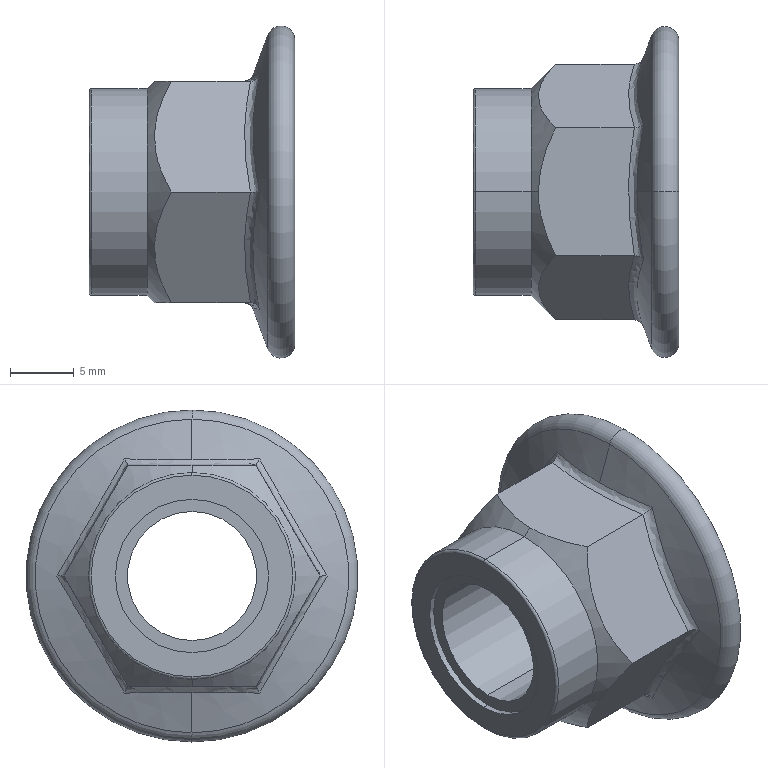Part | SolidWorks | features Cut 2, Revolution 2, Boss 1, Chamfer 1, Fillet 1 | 1 solid | 31 faces | box 16.1 x 26 x 26 mm | volume 3234 mm3 | plane 9 | cylinder 6 | cone 6 | spline 6 | torus 4 | commonest cylinder face diameters 10.106 x2 12 x2 16.2 x2
STEP:
#1=CARTESIAN_POINT('',(-16.1,0.,6.));
#2=VERTEX_POINT('',#1);
#3=CARTESIAN_POINT('',(-16.1,0.,-6.));
#4=VERTEX_POINT('',#3);
#5=CARTESIAN_POINT('',(-16.1,0.,0.));
#6=DIRECTION('',(1.,0.,0.));
#7=DIRECTION('',(0.,0.,-1.));
#8=AXIS2_PLACEMENT_3D('',#5,#6,#7);
#9=CIRCLE('',#8,6.);
#10=EDGE_CURVE('',#2,#4,#9,.T.);
#11=ORIENTED_EDGE('',*,*,#10,.F.);
#12=CARTESIAN_POINT('',(-15.647,0.,6.));
#13=VERTEX_POINT('',#12);
#14=CARTESIAN_POINT('',(0.,0.,6.));
#15=DIRECTION('',(1.,0.,0.));
#16=VECTOR('',#15,1000.);
#17=LINE('',#14,#16);
#18=EDGE_CURVE('',#2,#13,#17,.T.);
#19=ORIENTED_EDGE('',*,*,#18,.T.);
#20=CARTESIAN_POINT('',(-15.647,0.,-6.));
#21=VERTEX_POINT('',#20);
#22=CARTESIAN_POINT('',(-15.647,0.,0.));
#23=DIRECTION('',(1.,0.,0.));
#24=DIRECTION('',(0.,0.,-1.));
#25=AXIS2_PLACEMENT_3D('',#22,#23,#24);
#26=CIRCLE('',#25,6.);
#27=EDGE_CURVE('',#13,#21,#26,.T.);
#28=ORIENTED_EDGE('',*,*,#27,.T.);
#29=CARTESIAN_POINT('',(0.,0.,-6.));
#30=DIRECTION('',(1.,0.,0.));
#31=VECTOR('',#30,1000.);
#32=LINE('',#29,#31);
#33=EDGE_CURVE('',#4,#21,#32,.T.);
#34=ORIENTED_EDGE('',*,*,#33,.F.);
#35=EDGE_LOOP('',(#11,#19,#28,#34));
#36=FACE_OUTER_BOUND('',#35,.T.);
#37=CARTESIAN_POINT('',(0.,0.,0.));
#38=DIRECTION('',(1.,0.,0.));
#39=DIRECTION('',(0.,0.,-1.));
#40=AXIS2_PLACEMENT_3D('',#37,#38,#39);
#41=CYLINDRICAL_SURFACE('',#40,6.);
#42=ADVANCED_FACE('',(#36),#41,.F.);
#43=CARTESIAN_POINT('',(-16.1,0.,-7.9));
#44=VERTEX_POINT('',#43);
#45=CARTESIAN_POINT('',(-16.1,0.,7.9));
#46=VERTEX_POINT('',#45);
#47=CARTESIAN_POINT('',(-16.1,0.,0.));
#48=DIRECTION('',(1.,0.,0.));
#49=DIRECTION('',(0.,0.,-1.));
#50=AXIS2_PLACEMENT_3D('',#47,#48,#49);
#51=CIRCLE('',#50,7.9);
#52=EDGE_CURVE('',#44,#46,#51,.T.);
#53=ORIENTED_EDGE('',*,*,#52,.T.);
#54=CARTESIAN_POINT('',(-15.9,0.,8.1));
#55=VERTEX_POINT('',#54);
#56=CARTESIAN_POINT('',(-15.9,0.,7.9));
#57=DIRECTION('',(0.,1.,0.));
#58=DIRECTION('',(0.,0.,1.));
#59=AXIS2_PLACEMENT_3D('',#56,#57,#58);
#60=CIRCLE('',#59,0.2);
#61=EDGE_CURVE('',#46,#55,#60,.T.);
#62=ORIENTED_EDGE('',*,*,#61,.T.);
#63=CARTESIAN_POINT('',(-15.9,0.,-8.1));
#64=VERTEX_POINT('',#63);
#65=CARTESIAN_POINT('',(-15.9,0.,0.));
#66=DIRECTION('',(1.,0.,0.));
#67=DIRECTION('',(0.,0.,-1.));
#68=AXIS2_PLACEMENT_3D('',#65,#66,#67);
#69=CIRCLE('',#68,8.1);
#70=EDGE_CURVE('',#64,#55,#69,.T.);
#71=ORIENTED_EDGE('',*,*,#70,.F.);
#72=CARTESIAN_POINT('',(-15.9,0.,-7.9));
#73=DIRECTION('',(0.,-1.,0.));
#74=DIRECTION('',(0.,0.,-1.));
#75=AXIS2_PLACEMENT_3D('',#72,#73,#74);
#76=CIRCLE('',#75,0.2);
#77=EDGE_CURVE('',#44,#64,#76,.T.);
#78=ORIENTED_EDGE('',*,*,#77,.F.);
#79=EDGE_LOOP('',(#53,#62,#71,#78));
#80=FACE_OUTER_BOUND('',#79,.T.);
#81=CARTESIAN_POINT('',(-15.9,0.,0.));
#82=DIRECTION('',(1.,0.,0.));
#83=DIRECTION('',(0.,0.,-1.));
#84=AXIS2_PLACEMENT_3D('',#81,#82,#83);
#85=TOROIDAL_SURFACE('',#84,7.9,0.2);
#86=ADVANCED_FACE('',(#80),#85,.T.);
#87=ORIENTED_EDGE('',*,*,#70,.T.);
#88=CARTESIAN_POINT('',(-11.57,0.,8.1));
#89=VERTEX_POINT('',#88);
#90=CARTESIAN_POINT('',(0.,0.,8.1));
#91=DIRECTION('',(1.,0.,0.));
#92=VECTOR('',#91,1000.);
#93=LINE('',#90,#92);
#94=EDGE_CURVE('',#55,#89,#93,.T.);
#95=ORIENTED_EDGE('',*,*,#94,.T.);
#96=CARTESIAN_POINT('',(-11.57,0.,-8.1));
#97=VERTEX_POINT('',#96);
#98=CARTESIAN_POINT('',(-11.57,0.,0.));
#99=DIRECTION('',(-1.,0.,0.));
#100=DIRECTION('',(0.,0.,1.));
#101=AXIS2_PLACEMENT_3D('',#98,#99,#100);
#102=CIRCLE('',#101,8.1);
#103=EDGE_CURVE('',#89,#97,#102,.T.);
#104=ORIENTED_EDGE('',*,*,#103,.T.);
#105=CARTESIAN_POINT('',(0.,0.,-8.1));
#106=DIRECTION('',(1.,0.,0.));
#107=VECTOR('',#106,1000.);
#108=LINE('',#105,#107);
#109=EDGE_CURVE('',#64,#97,#108,.T.);
#110=ORIENTED_EDGE('',*,*,#109,.F.);
#111=EDGE_LOOP('',(#87,#95,#104,#110));
#112=FACE_OUTER_BOUND('',#111,.T.);
#113=CARTESIAN_POINT('',(0.,0.,0.));
#114=DIRECTION('',(1.,0.,0.));
#115=DIRECTION('',(0.,0.,-1.));
#116=AXIS2_PLACEMENT_3D('',#113,#114,#115);
#117=CYLINDRICAL_SURFACE('',#116,8.1);
#118=ADVANCED_FACE('',(#112),#117,.T.);
#119=CARTESIAN_POINT('',(-11.57,0.,0.));
#120=DIRECTION('',(-1.,0.,0.));
#121=DIRECTION('',(0.,0.,1.));
#122=AXIS2_PLACEMENT_3D('',#119,#120,#121);
#123=CIRCLE('',#122,8.1);
#124=EDGE_CURVE('',#97,#89,#123,.T.);
#125=ORIENTED_EDGE('',*,*,#124,.F.);
#126=CARTESIAN_POINT('',(-10.997,0.,-8.673));
#127=VERTEX_POINT('',#126);
#128=CARTESIAN_POINT('',(-11.57,0.,-8.1));
#129=DIRECTION('',(0.7071,0.,-0.7071));
#130=VECTOR('',#129,1000.);
#131=LINE('',#128,#130);
#132=EDGE_CURVE('',#97,#127,#131,.T.);
#133=ORIENTED_EDGE('',*,*,#132,.T.);
#134=CARTESIAN_POINT('',(-9.655,-5.007,-8.673));
#135=VERTEX_POINT('',#134);
#136=CARTESIAN_POINT('',(-10.997,0.,-8.673));
#137=CARTESIAN_POINT('',(-10.997,-0.2199,-8.673));
#138=CARTESIAN_POINT('',(-10.988,-0.4408,-8.673));
#139=CARTESIAN_POINT('',(-10.955,-0.877,-8.673));
#140=CARTESIAN_POINT('',(-10.931,-1.093,-8.673));
#141=CARTESIAN_POINT('',(-10.835,-1.738,-8.673));
#142=CARTESIAN_POINT('',(-10.741,-2.161,-8.673));
#143=CARTESIAN_POINT('',(-10.503,-2.996,-8.673));
#144=CARTESIAN_POINT('',(-10.358,-3.409,-8.673));
#145=CARTESIAN_POINT('',(-10.03,-4.223,-8.673));
#146=CARTESIAN_POINT('',(-9.849,-4.619,-8.673));
#147=CARTESIAN_POINT('',(-9.655,-5.007,-8.673));
#148=B_SPLINE_CURVE_WITH_KNOTS('',3,(#136,#137,#138,#139,#140,#141,#142,#143,#144,#145,#146,#147),.UNSPECIFIED.,.F.,.F.,(4,2,2,2,2,4),(0.01051,0.01116,0.01181,0.01311,0.0144,0.0157),.UNSPECIFIED.);
#149=EDGE_CURVE('',#127,#135,#148,.T.);
#150=ORIENTED_EDGE('',*,*,#149,.T.);
#151=CARTESIAN_POINT('',(-9.655,-10.015,0.));
#152=VERTEX_POINT('',#151);
#153=CARTESIAN_POINT('',(-9.655,-5.007,-8.673));
#154=CARTESIAN_POINT('',(-10.046,-5.399,-7.996));
#155=CARTESIAN_POINT('',(-10.379,-5.799,-7.303));
#156=CARTESIAN_POINT('',(-10.735,-6.42,-6.226));
#157=CARTESIAN_POINT('',(-10.83,-6.631,-5.861));
#158=CARTESIAN_POINT('',(-10.961,-7.062,-5.115));
#159=CARTESIAN_POINT('',(-10.996,-7.283,-4.731));
#160=CARTESIAN_POINT('',(-10.999,-7.939,-3.595));
#161=CARTESIAN_POINT('',(-10.866,-8.369,-2.851));
#162=CARTESIAN_POINT('',(-10.386,-9.216,-1.384));
#163=CARTESIAN_POINT('',(-10.049,-9.621,-0.6817));
#164=CARTESIAN_POINT('',(-9.655,-10.015,0.));
#165=B_SPLINE_CURVE_WITH_KNOTS('',3,(#153,#154,#155,#156,#157,#158,#159,#160,#161,#162,#163,#164),.UNSPECIFIED.,.F.,.F.,(4,2,2,2,2,4),(0.000000254,0.002587,0.00388,0.005173,0.007759,0.01035),.UNSPECIFIED.);
#166=EDGE_CURVE('',#135,#152,#165,.T.);
#167=ORIENTED_EDGE('',*,*,#166,.T.);
#168=CARTESIAN_POINT('',(-9.655,-5.008,8.673));
#169=VERTEX_POINT('',#168);
#170=CARTESIAN_POINT('',(-9.655,-10.015,0.));
#171=CARTESIAN_POINT('',(-10.046,-9.624,0.6777));
#172=CARTESIAN_POINT('',(-10.379,-9.224,1.371));
#173=CARTESIAN_POINT('',(-10.735,-8.602,2.447));
#174=CARTESIAN_POINT('',(-10.83,-8.391,2.812));
#175=CARTESIAN_POINT('',(-10.961,-7.961,3.558));
#176=CARTESIAN_POINT('',(-10.996,-7.739,3.942));
#177=CARTESIAN_POINT('',(-10.999,-7.083,5.078));
#178=CARTESIAN_POINT('',(-10.866,-6.654,5.822));
#179=CARTESIAN_POINT('',(-10.386,-5.806,7.29));
#180=CARTESIAN_POINT('',(-10.049,-5.401,7.992));
#181=CARTESIAN_POINT('',(-9.655,-5.008,8.673));
#182=B_SPLINE_CURVE_WITH_KNOTS('',3,(#170,#171,#172,#173,#174,#175,#176,#177,#178,#179,#180,#181),.UNSPECIFIED.,.F.,.F.,(4,2,2,2,2,4),(0.000000254,0.002587,0.00388,0.005173,0.007759,0.01035),.UNSPECIFIED.);
#183=EDGE_CURVE('',#152,#169,#182,.T.);
#184=ORIENTED_EDGE('',*,*,#183,.T.);
#185=CARTESIAN_POINT('',(-10.997,0.,8.673));
#186=VERTEX_POINT('',#185);
#187=CARTESIAN_POINT('',(-9.655,-5.008,8.673));
#188=CARTESIAN_POINT('',(-9.849,-4.619,8.673));
#189=CARTESIAN_POINT('',(-10.03,-4.223,8.673));
#190=CARTESIAN_POINT('',(-10.358,-3.409,8.673));
#191=CARTESIAN_POINT('',(-10.503,-2.996,8.673));
#192=CARTESIAN_POINT('',(-10.741,-2.161,8.673));
#193=CARTESIAN_POINT('',(-10.835,-1.738,8.673));
#194=CARTESIAN_POINT('',(-10.931,-1.093,8.673));
#195=CARTESIAN_POINT('',(-10.955,-0.877,8.673));
#196=CARTESIAN_POINT('',(-10.988,-0.4408,8.673));
#197=CARTESIAN_POINT('',(-10.997,-0.2199,8.673));
#198=CARTESIAN_POINT('',(-10.997,0.,8.673));
#199=B_SPLINE_CURVE_WITH_KNOTS('',3,(#187,#188,#189,#190,#191,#192,#193,#194,#195,#196,#197,#198),.UNSPECIFIED.,.F.,.F.,(4,2,2,2,2,4),(0.006513,0.007811,0.009108,0.01041,0.01105,0.0117),.UNSPECIFIED.);
#200=EDGE_CURVE('',#169,#186,#199,.T.);
#201=ORIENTED_EDGE('',*,*,#200,.T.);
#202=CARTESIAN_POINT('',(-11.57,0.,8.1));
#203=DIRECTION('',(0.7071,0.,0.7071));
#204=VECTOR('',#203,1000.);
#205=LINE('',#202,#204);
#206=EDGE_CURVE('',#89,#186,#205,.T.);
#207=ORIENTED_EDGE('',*,*,#206,.F.);
#208=EDGE_LOOP('',(#125,#133,#150,#167,#184,#201,#207));
#209=FACE_OUTER_BOUND('',#208,.T.);
#210=CARTESIAN_POINT('',(-11.57,0.,0.));
#211=DIRECTION('',(1.,0.,0.));
#212=DIRECTION('',(0.,0.,1.));
#213=AXIS2_PLACEMENT_3D('',#210,#211,#212);
#214=CONICAL_SURFACE('',#213,8.1,0.7854);
#215=ADVANCED_FACE('',(#209),#214,.T.);
#216=CARTESIAN_POINT('',(-1.447,0.,5.053));
#217=VERTEX_POINT('',#216);
#218=CARTESIAN_POINT('',(-1.447,0.,-5.053));
#219=VERTEX_POINT('',#218);
#220=CARTESIAN_POINT('',(-1.447,0.,0.));
#221=DIRECTION('',(1.,0.,0.));
#222=DIRECTION('',(0.,0.,1.));
#223=AXIS2_PLACEMENT_3D('',#220,#221,#222);
#224=CIRCLE('',#223,5.053);
#225=EDGE_CURVE('',#217,#219,#224,.T.);
#226=ORIENTED_EDGE('',*,*,#225,.F.);
#227=CARTESIAN_POINT('',(0.,0.,6.5));
#228=VERTEX_POINT('',#227);
#229=CARTESIAN_POINT('',(0.,0.,6.5));
#230=DIRECTION('',(0.7071,0.,0.7071));
#231=VECTOR('',#230,1000.);
#232=LINE('',#229,#231);
#233=EDGE_CURVE('',#217,#228,#232,.T.);
#234=ORIENTED_EDGE('',*,*,#233,.T.);
#235=CARTESIAN_POINT('',(0.,0.,-6.5));
#236=VERTEX_POINT('',#235);
#237=CARTESIAN_POINT('',(0.,0.,0.));
#238=DIRECTION('',(-1.,0.,0.));
#239=DIRECTION('',(0.,0.,1.));
#240=AXIS2_PLACEMENT_3D('',#237,#238,#239);
#241=CIRCLE('',#240,6.5);
#242=EDGE_CURVE('',#236,#228,#241,.T.);
#243=ORIENTED_EDGE('',*,*,#242,.F.);
#244=CARTESIAN_POINT('',(0.,0.,-6.5));
#245=DIRECTION('',(0.7071,0.,-0.7071));
#246=VECTOR('',#245,1000.);
#247=LINE('',#244,#246);
#248=EDGE_CURVE('',#219,#236,#247,.T.);
#249=ORIENTED_EDGE('',*,*,#248,.F.);
#250=EDGE_LOOP('',(#226,#234,#243,#249));
#251=FACE_OUTER_BOUND('',#250,.T.);
#252=CARTESIAN_POINT('',(0.,0.,0.));
#253=DIRECTION('',(1.,0.,0.));
#254=DIRECTION('',(0.,0.,-1.));
#255=AXIS2_PLACEMENT_3D('',#252,#253,#254);
#256=CONICAL_SURFACE('',#255,6.5,0.7854);
#257=ADVANCED_FACE('',(#251),#256,.F.);
#258=ORIENTED_EDGE('',*,*,#225,.T.);
#259=CARTESIAN_POINT('',(-15.647,0.,-5.053));
#260=VERTEX_POINT('',#259);
#261=CARTESIAN_POINT('',(0.,0.,-5.053));
#262=DIRECTION('',(-1.,0.,0.));
#263=VECTOR('',#262,1000.);
#264=LINE('',#261,#263);
#265=EDGE_CURVE('',#219,#260,#264,.T.);
#266=ORIENTED_EDGE('',*,*,#265,.T.);
#267=CARTESIAN_POINT('',(-15.647,0.,5.053));
#268=VERTEX_POINT('',#267);
#269=CARTESIAN_POINT('',(-15.647,0.,0.));
#270=DIRECTION('',(1.,0.,0.));
#271=DIRECTION('',(0.,0.,-1.));
#272=AXIS2_PLACEMENT_3D('',#269,#270,#271);
#273=CIRCLE('',#272,5.053);
#274=EDGE_CURVE('',#268,#260,#273,.T.);
#275=ORIENTED_EDGE('',*,*,#274,.F.);
#276=CARTESIAN_POINT('',(0.,0.,5.053));
#277=DIRECTION('',(-1.,0.,0.));
#278=VECTOR('',#277,1000.);
#279=LINE('',#276,#278);
#280=EDGE_CURVE('',#217,#268,#279,.T.);
#281=ORIENTED_EDGE('',*,*,#280,.F.);
#282=EDGE_LOOP('',(#258,#266,#275,#281));
#283=FACE_OUTER_BOUND('',#282,.T.);
#284=CARTESIAN_POINT('',(0.,0.,0.));
#285=DIRECTION('',(-1.,0.,0.));
#286=DIRECTION('',(0.,0.,1.));
#287=AXIS2_PLACEMENT_3D('',#284,#285,#286);
#288=CYLINDRICAL_SURFACE('',#287,5.053);
#289=ADVANCED_FACE('',(#283),#288,.F.);
#290=CARTESIAN_POINT('',(0.,0.,11.9));
#291=VERTEX_POINT('',#290);
#292=CARTESIAN_POINT('',(0.,0.,-11.9));
#293=VERTEX_POINT('',#292);
#294=CARTESIAN_POINT('',(0.,0.,0.));
#295=DIRECTION('',(-1.,0.,0.));
#296=DIRECTION('',(0.,0.,1.));
#297=AXIS2_PLACEMENT_3D('',#294,#295,#296);
#298=CIRCLE('',#297,11.9);
#299=EDGE_CURVE('',#291,#293,#298,.T.);
#300=ORIENTED_EDGE('',*,*,#299,.T.);
#301=CARTESIAN_POINT('',(-2.134,0.,-12.276));
#302=VERTEX_POINT('',#301);
#303=CARTESIAN_POINT('',(-1.1,0.,-11.9));
#304=DIRECTION('',(0.,1.,0.));
#305=DIRECTION('',(0.,0.,1.));
#306=AXIS2_PLACEMENT_3D('',#303,#304,#305);
#307=CIRCLE('',#306,1.1);
#308=EDGE_CURVE('',#293,#302,#307,.T.);
#309=ORIENTED_EDGE('',*,*,#308,.T.);
#310=CARTESIAN_POINT('',(-2.134,0.,12.276));
#311=VERTEX_POINT('',#310);
#312=CARTESIAN_POINT('',(-2.134,0.,0.));
#313=DIRECTION('',(-1.,0.,0.));
#314=DIRECTION('',(0.,0.,1.));
#315=AXIS2_PLACEMENT_3D('',#312,#313,#314);
#316=CIRCLE('',#315,12.276);
#317=EDGE_CURVE('',#311,#302,#316,.T.);
#318=ORIENTED_EDGE('',*,*,#317,.F.);
#319=CARTESIAN_POINT('',(-1.1,0.,11.9));
#320=DIRECTION('',(0.,-1.,0.));
#321=DIRECTION('',(0.,0.,-1.));
#322=AXIS2_PLACEMENT_3D('',#319,#320,#321);
#323=CIRCLE('',#322,1.1);
#324=EDGE_CURVE('',#291,#311,#323,.T.);
#325=ORIENTED_EDGE('',*,*,#324,.F.);
#326=EDGE_LOOP('',(#300,#309,#318,#325));
#327=FACE_OUTER_BOUND('',#326,.T.);
#328=CARTESIAN_POINT('',(-1.1,0.,0.));
#329=DIRECTION('',(-1.,0.,0.));
#330=DIRECTION('',(0.,0.,1.));
#331=AXIS2_PLACEMENT_3D('',#328,#329,#330);
#332=TOROIDAL_SURFACE('',#331,11.9,1.1);
#333=ADVANCED_FACE('',(#327),#332,.T.);
#334=CARTESIAN_POINT('',(-2.75,5.292,9.166));
#335=VERTEX_POINT('',#334);
#336=CARTESIAN_POINT('',(-3.277,0.,9.134));
#337=VERTEX_POINT('',#336);
#338=CARTESIAN_POINT('',(-2.75,5.292,9.166));
#339=CARTESIAN_POINT('',(-2.911,4.417,9.157));
#340=CARTESIAN_POINT('',(-3.044,3.54,9.149));
#341=CARTESIAN_POINT('',(-3.228,1.777,9.137));
#342=CARTESIAN_POINT('',(-3.277,0.8908,9.134));
#343=CARTESIAN_POINT('',(-3.277,0.,9.134));
#344=B_SPLINE_CURVE_WITH_KNOTS('',3,(#338,#339,#340,#341,#342,#343),.UNSPECIFIED.,.F.,.F.,(4,2,4),(0.,0.002659,0.005318),.UNSPECIFIED.);
#345=EDGE_CURVE('',#335,#337,#344,.T.);
#346=ORIENTED_EDGE('',*,*,#345,.T.);
#347=CARTESIAN_POINT('',(-2.134,0.,12.276));
#348=DIRECTION('',(0.342,0.,0.9397));
#349=VECTOR('',#348,1000.);
#350=LINE('',#347,#349);
#351=EDGE_CURVE('',#337,#311,#350,.T.);
#352=ORIENTED_EDGE('',*,*,#351,.T.);
#353=ORIENTED_EDGE('',*,*,#317,.T.);
#354=CARTESIAN_POINT('',(-3.277,0.,-9.134));
#355=VERTEX_POINT('',#354);
#356=CARTESIAN_POINT('',(-2.134,0.,-12.276));
#357=DIRECTION('',(0.342,0.,-0.9397));
#358=VECTOR('',#357,1000.);
#359=LINE('',#356,#358);
#360=EDGE_CURVE('',#355,#302,#359,.T.);
#361=ORIENTED_EDGE('',*,*,#360,.F.);
#362=CARTESIAN_POINT('',(-2.75,5.292,-9.166));
#363=VERTEX_POINT('',#362);
#364=CARTESIAN_POINT('',(-3.277,0.,-9.134));
#365=CARTESIAN_POINT('',(-3.277,0.8884,-9.134));
#366=CARTESIAN_POINT('',(-3.228,1.775,-9.137));
#367=CARTESIAN_POINT('',(-3.044,3.541,-9.149));
#368=CARTESIAN_POINT('',(-2.911,4.419,-9.157));
#369=CARTESIAN_POINT('',(-2.75,5.292,-9.166));
#370=B_SPLINE_CURVE_WITH_KNOTS('',3,(#364,#365,#366,#367,#368,#369),.UNSPECIFIED.,.F.,.F.,(4,2,4),(0.005318,0.00797,0.01062),.UNSPECIFIED.);
#371=EDGE_CURVE('',#355,#363,#370,.T.);
#372=ORIENTED_EDGE('',*,*,#371,.T.);
#373=CARTESIAN_POINT('',(-2.75,10.584,0.));
#374=VERTEX_POINT('',#373);
#375=CARTESIAN_POINT('',(-2.75,5.292,-9.166));
#376=CARTESIAN_POINT('',(-2.911,5.721,-8.405));
#377=CARTESIAN_POINT('',(-3.044,6.152,-7.642));
#378=CARTESIAN_POINT('',(-3.227,7.023,-6.111));
#379=CARTESIAN_POINT('',(-3.277,7.462,-5.344));
#380=CARTESIAN_POINT('',(-3.278,8.351,-3.803));
#381=CARTESIAN_POINT('',(-3.228,8.798,-3.036));
#382=CARTESIAN_POINT('',(-3.045,9.693,-1.51));
#383=CARTESIAN_POINT('',(-2.911,10.139,-0.753));
#384=CARTESIAN_POINT('',(-2.75,10.584,0.));
#385=B_SPLINE_CURVE_WITH_KNOTS('',3,(#375,#376,#377,#378,#379,#380,#381,#382,#383,#384),.UNSPECIFIED.,.F.,.F.,(4,2,2,2,4),(0.,0.002656,0.005311,0.007967,0.01062),.UNSPECIFIED.);
#386=EDGE_CURVE('',#363,#374,#385,.T.);
#387=ORIENTED_EDGE('',*,*,#386,.T.);
#388=CARTESIAN_POINT('',(-2.75,10.584,0.));
#389=CARTESIAN_POINT('',(-2.911,10.14,0.7522));
#390=CARTESIAN_POINT('',(-3.044,9.695,1.507));
#391=CARTESIAN_POINT('',(-3.227,8.804,3.026));
#392=CARTESIAN_POINT('',(-3.277,8.359,3.79));
#393=CARTESIAN_POINT('',(-3.278,7.469,5.331));
#394=CARTESIAN_POINT('',(-3.228,7.028,6.101));
#395=CARTESIAN_POINT('',(-3.045,6.154,7.639));
#396=CARTESIAN_POINT('',(-2.911,5.722,8.404));
#397=CARTESIAN_POINT('',(-2.75,5.292,9.166));
#398=B_SPLINE_CURVE_WITH_KNOTS('',3,(#388,#389,#390,#391,#392,#393,#394,#395,#396,#397),.UNSPECIFIED.,.F.,.F.,(4,2,2,2,4),(0.,0.002656,0.005311,0.007967,0.01062),.UNSPECIFIED.);
#399=EDGE_CURVE('',#374,#335,#398,.T.);
#400=ORIENTED_EDGE('',*,*,#399,.T.);
#401=EDGE_LOOP('',(#346,#352,#353,#361,#372,#387,#400));
#402=FACE_OUTER_BOUND('',#401,.T.);
#403=CARTESIAN_POINT('',(-2.134,0.,0.));
#404=DIRECTION('',(1.,0.,0.));
#405=DIRECTION('',(0.,0.,-1.));
#406=AXIS2_PLACEMENT_3D('',#403,#404,#405);
#407=CONICAL_SURFACE('',#406,12.276,1.222);
#408=ADVANCED_FACE('',(#402),#407,.T.);
#409=CARTESIAN_POINT('',(-9.655,5.008,8.673));
#410=VERTEX_POINT('',#409);
#411=CARTESIAN_POINT('',(-3.479,5.008,8.673));
#412=VERTEX_POINT('',#411);
#413=CARTESIAN_POINT('',(-11.57,5.008,8.673));
#414=DIRECTION('',(1.,0.,0.));
#415=VECTOR('',#414,1000.);
#416=LINE('',#413,#415);
#417=EDGE_CURVE('',#410,#412,#416,.T.);
#418=ORIENTED_EDGE('',*,*,#417,.T.);
#419=CARTESIAN_POINT('',(-3.479,10.015,0.));
#420=VERTEX_POINT('',#419);
#421=CARTESIAN_POINT('',(-3.479,5.008,8.673));
#422=CARTESIAN_POINT('',(-3.621,5.422,7.956));
#423=CARTESIAN_POINT('',(-3.736,5.837,7.236));
#424=CARTESIAN_POINT('',(-3.893,6.672,5.791));
#425=CARTESIAN_POINT('',(-3.935,7.09,5.065));
#426=CARTESIAN_POINT('',(-3.935,7.932,3.608));
#427=CARTESIAN_POINT('',(-3.893,8.351,2.882));
#428=CARTESIAN_POINT('',(-3.736,9.185,1.437));
#429=CARTESIAN_POINT('',(-3.621,9.601,0.7176));
#430=CARTESIAN_POINT('',(-3.479,10.015,0.));
#431=B_SPLINE_CURVE_WITH_KNOTS('',3,(#421,#422,#423,#424,#425,#426,#427,#428,#429,#430),.UNSPECIFIED.,.F.,.F.,(4,2,2,2,4),(0.,0.002514,0.005028,0.007542,0.01006),.UNSPECIFIED.);
#432=EDGE_CURVE('',#412,#420,#431,.T.);
#433=ORIENTED_EDGE('',*,*,#432,.T.);
#434=CARTESIAN_POINT('',(-9.655,10.015,0.));
#435=VERTEX_POINT('',#434);
#436=CARTESIAN_POINT('',(-11.57,10.015,0.));
#437=DIRECTION('',(1.,0.,0.));
#438=VECTOR('',#437,1000.);
#439=LINE('',#436,#438);
#440=EDGE_CURVE('',#435,#420,#439,.T.);
#441=ORIENTED_EDGE('',*,*,#440,.F.);
#442=CARTESIAN_POINT('',(-9.655,5.008,8.673));
#443=CARTESIAN_POINT('',(-10.046,5.399,7.996));
#444=CARTESIAN_POINT('',(-10.379,5.799,7.303));
#445=CARTESIAN_POINT('',(-10.735,6.42,6.226));
#446=CARTESIAN_POINT('',(-10.83,6.631,5.861));
#447=CARTESIAN_POINT('',(-10.961,7.062,5.115));
#448=CARTESIAN_POINT('',(-10.996,7.283,4.731));
#449=CARTESIAN_POINT('',(-10.999,7.939,3.595));
#450=CARTESIAN_POINT('',(-10.866,8.369,2.851));
#451=CARTESIAN_POINT('',(-10.386,9.216,1.384));
#452=CARTESIAN_POINT('',(-10.049,9.621,0.6817));
#453=CARTESIAN_POINT('',(-9.655,10.015,0.));
#454=B_SPLINE_CURVE_WITH_KNOTS('',3,(#442,#443,#444,#445,#446,#447,#448,#449,#450,#451,#452,#453),.UNSPECIFIED.,.F.,.F.,(4,2,2,2,2,4),(0.000000254,0.002587,0.00388,0.005173,0.007759,0.01035),.UNSPECIFIED.);
#455=EDGE_CURVE('',#410,#435,#454,.T.);
#456=ORIENTED_EDGE('',*,*,#455,.F.);
#457=EDGE_LOOP('',(#418,#433,#441,#456));
#458=FACE_OUTER_BOUND('',#457,.T.);
#459=CARTESIAN_POINT('',(-11.57,5.008,8.673));
#460=DIRECTION('',(0.,-0.866,-0.5));
#461=DIRECTION('',(0.,0.5,-0.866));
#462=AXIS2_PLACEMENT_3D('',#459,#460,#461);
#463=PLANE('',#462);
#464=ADVANCED_FACE('',(#458),#463,.F.);
#465=ORIENTED_EDGE('',*,*,#440,.T.);
#466=CARTESIAN_POINT('',(-3.479,5.008,-8.673));
#467=VERTEX_POINT('',#466);
#468=CARTESIAN_POINT('',(-3.479,10.015,0.));
#469=CARTESIAN_POINT('',(-3.621,9.601,-0.7176));
#470=CARTESIAN_POINT('',(-3.736,9.185,-1.437));
#471=CARTESIAN_POINT('',(-3.893,8.351,-2.882));
#472=CARTESIAN_POINT('',(-3.935,7.932,-3.608));
#473=CARTESIAN_POINT('',(-3.935,7.09,-5.065));
#474=CARTESIAN_POINT('',(-3.893,6.672,-5.791));
#475=CARTESIAN_POINT('',(-3.736,5.837,-7.236));
#476=CARTESIAN_POINT('',(-3.621,5.422,-7.956));
#477=CARTESIAN_POINT('',(-3.479,5.008,-8.673));
#478=B_SPLINE_CURVE_WITH_KNOTS('',3,(#468,#469,#470,#471,#472,#473,#474,#475,#476,#477),.UNSPECIFIED.,.F.,.F.,(4,2,2,2,4),(0.,0.002514,0.005028,0.007542,0.01006),.UNSPECIFIED.);
#479=EDGE_CURVE('',#420,#467,#478,.T.);
#480=ORIENTED_EDGE('',*,*,#479,.T.);
#481=CARTESIAN_POINT('',(-9.655,5.008,-8.673));
#482=VERTEX_POINT('',#481);
#483=CARTESIAN_POINT('',(-11.57,5.008,-8.673));
#484=DIRECTION('',(1.,0.,0.));
#485=VECTOR('',#484,1000.);
#486=LINE('',#483,#485);
#487=EDGE_CURVE('',#482,#467,#486,.T.);
#488=ORIENTED_EDGE('',*,*,#487,.F.);
#489=CARTESIAN_POINT('',(-9.655,10.015,0.));
#490=CARTESIAN_POINT('',(-10.046,9.624,-0.6777));
#491=CARTESIAN_POINT('',(-10.379,9.224,-1.371));
#492=CARTESIAN_POINT('',(-10.735,8.602,-2.447));
#493=CARTESIAN_POINT('',(-10.83,8.391,-2.812));
#494=CARTESIAN_POINT('',(-10.961,7.961,-3.558));
#495=CARTESIAN_POINT('',(-10.996,7.739,-3.942));
#496=CARTESIAN_POINT('',(-10.999,7.083,-5.078));
#497=CARTESIAN_POINT('',(-10.866,6.654,-5.822));
#498=CARTESIAN_POINT('',(-10.386,5.806,-7.29));
#499=CARTESIAN_POINT('',(-10.049,5.401,-7.992));
#500=CARTESIAN_POINT('',(-9.655,5.008,-8.673));
#501=B_SPLINE_CURVE_WITH_KNOTS('',3,(#489,#490,#491,#492,#493,#494,#495,#496,#497,#498,#499,#500),.UNSPECIFIED.,.F.,.F.,(4,2,2,2,2,4),(0.000000254,0.002587,0.00388,0.005173,0.007759,0.01035),.UNSPECIFIED.);
#502=EDGE_CURVE('',#435,#482,#501,.T.);
#503=ORIENTED_EDGE('',*,*,#502,.F.);
#504=EDGE_LOOP('',(#465,#480,#488,#503));
#505=FACE_OUTER_BOUND('',#504,.T.);
#506=CARTESIAN_POINT('',(-11.57,10.015,0.));
#507=DIRECTION('',(0.,-0.866,0.5));
#508=DIRECTION('',(0.,-0.5,-0.866));
#509=AXIS2_PLACEMENT_3D('',#506,#507,#508);
#510=PLANE('',#509);
#511=ADVANCED_FACE('',(#505),#510,.F.);
#512=ORIENTED_EDGE('',*,*,#487,.T.);
#513=CARTESIAN_POINT('',(-3.479,-5.007,-8.673));
#514=VERTEX_POINT('',#513);
#515=CARTESIAN_POINT('',(-3.479,5.008,-8.673));
#516=CARTESIAN_POINT('',(-3.621,4.179,-8.673));
#517=CARTESIAN_POINT('',(-3.736,3.348,-8.673));
#518=CARTESIAN_POINT('',(-3.893,1.679,-8.673));
#519=CARTESIAN_POINT('',(-3.935,0.8414,-8.673));
#520=CARTESIAN_POINT('',(-3.935,-0.8416,-8.673));
#521=CARTESIAN_POINT('',(-3.893,-1.679,-8.673));
#522=CARTESIAN_POINT('',(-3.736,-3.348,-8.673));
#523=CARTESIAN_POINT('',(-3.621,-4.179,-8.673));
#524=CARTESIAN_POINT('',(-3.479,-5.007,-8.673));
#525=B_SPLINE_CURVE_WITH_KNOTS('',3,(#515,#516,#517,#518,#519,#520,#521,#522,#523,#524),.UNSPECIFIED.,.F.,.F.,(4,2,2,2,4),(0.,0.002514,0.005028,0.007542,0.01006),.UNSPECIFIED.);
#526=EDGE_CURVE('',#467,#514,#525,.T.);
#527=ORIENTED_EDGE('',*,*,#526,.T.);
#528=CARTESIAN_POINT('',(-11.57,-5.007,-8.673));
#529=DIRECTION('',(1.,0.,0.));
#530=VECTOR('',#529,1000.);
#531=LINE('',#528,#530);
#532=EDGE_CURVE('',#135,#514,#531,.T.);
#533=ORIENTED_EDGE('',*,*,#532,.F.);
#534=ORIENTED_EDGE('',*,*,#149,.F.);
#535=CARTESIAN_POINT('',(-9.655,5.008,-8.673));
#536=CARTESIAN_POINT('',(-9.849,4.62,-8.673));
#537=CARTESIAN_POINT('',(-10.03,4.225,-8.673));
#538=CARTESIAN_POINT('',(-10.356,3.415,-8.673));
#539=CARTESIAN_POINT('',(-10.502,2.997,-8.673));
#540=CARTESIAN_POINT('',(-10.861,1.738,-8.673));
#541=CARTESIAN_POINT('',(-10.997,0.8806,-8.673));
#542=CARTESIAN_POINT('',(-10.997,0.,-8.673));
#543=B_SPLINE_CURVE_WITH_KNOTS('',3,(#535,#536,#537,#538,#539,#540,#541,#542),.UNSPECIFIED.,.F.,.F.,(4,2,2,4),(0.005323,0.00662,0.007918,0.01051),.UNSPECIFIED.);
#544=EDGE_CURVE('',#482,#127,#543,.T.);
#545=ORIENTED_EDGE('',*,*,#544,.F.);
#546=EDGE_LOOP('',(#512,#527,#533,#534,#545));
#547=FACE_OUTER_BOUND('',#546,.T.);
#548=CARTESIAN_POINT('',(-11.57,5.008,-8.673));
#549=DIRECTION('',(0.,0.,1.));
#550=DIRECTION('',(0.,-1.,0.));
#551=AXIS2_PLACEMENT_3D('',#548,#549,#550);
#552=PLANE('',#551);
#553=ADVANCED_FACE('',(#547),#552,.F.);
#554=ORIENTED_EDGE('',*,*,#532,.T.);
#555=CARTESIAN_POINT('',(-3.479,-10.015,0.));
#556=VERTEX_POINT('',#555);
#557=CARTESIAN_POINT('',(-3.479,-5.007,-8.673));
#558=CARTESIAN_POINT('',(-3.621,-5.422,-7.956));
#559=CARTESIAN_POINT('',(-3.736,-5.837,-7.236));
#560=CARTESIAN_POINT('',(-3.893,-6.672,-5.791));
#561=CARTESIAN_POINT('',(-3.935,-7.09,-5.065));
#562=CARTESIAN_POINT('',(-3.935,-7.932,-3.608));
#563=CARTESIAN_POINT('',(-3.893,-8.351,-2.882));
#564=CARTESIAN_POINT('',(-3.736,-9.185,-1.437));
#565=CARTESIAN_POINT('',(-3.621,-9.601,-0.7176));
#566=CARTESIAN_POINT('',(-3.479,-10.015,0.));
#567=B_SPLINE_CURVE_WITH_KNOTS('',3,(#557,#558,#559,#560,#561,#562,#563,#564,#565,#566),.UNSPECIFIED.,.F.,.F.,(4,2,2,2,4),(0.,0.002514,0.005028,0.007542,0.01006),.UNSPECIFIED.);
#568=EDGE_CURVE('',#514,#556,#567,.T.);
#569=ORIENTED_EDGE('',*,*,#568,.T.);
#570=CARTESIAN_POINT('',(-11.57,-10.015,0.));
#571=DIRECTION('',(1.,0.,0.));
#572=VECTOR('',#571,1000.);
#573=LINE('',#570,#572);
#574=EDGE_CURVE('',#152,#556,#573,.T.);
#575=ORIENTED_EDGE('',*,*,#574,.F.);
#576=ORIENTED_EDGE('',*,*,#166,.F.);
#577=EDGE_LOOP('',(#554,#569,#575,#576));
#578=FACE_OUTER_BOUND('',#577,.T.);
#579=CARTESIAN_POINT('',(-11.57,-5.007,-8.673));
#580=DIRECTION('',(0.,0.866,0.5));
#581=DIRECTION('',(0.,-0.5,0.866));
#582=AXIS2_PLACEMENT_3D('',#579,#580,#581);
#583=PLANE('',#582);
#584=ADVANCED_FACE('',(#578),#583,.F.);
#585=ORIENTED_EDGE('',*,*,#574,.T.);
#586=CARTESIAN_POINT('',(-3.479,-5.008,8.673));
#587=VERTEX_POINT('',#586);
#588=CARTESIAN_POINT('',(-3.479,-10.015,0.));
#589=CARTESIAN_POINT('',(-3.621,-9.601,0.7176));
#590=CARTESIAN_POINT('',(-3.736,-9.185,1.437));
#591=CARTESIAN_POINT('',(-3.893,-8.351,2.882));
#592=CARTESIAN_POINT('',(-3.935,-7.932,3.608));
#593=CARTESIAN_POINT('',(-3.935,-7.09,5.065));
#594=CARTESIAN_POINT('',(-3.893,-6.672,5.791));
#595=CARTESIAN_POINT('',(-3.736,-5.837,7.236));
#596=CARTESIAN_POINT('',(-3.621,-5.422,7.956));
#597=CARTESIAN_POINT('',(-3.479,-5.008,8.673));
#598=B_SPLINE_CURVE_WITH_KNOTS('',3,(#588,#589,#590,#591,#592,#593,#594,#595,#596,#597),.UNSPECIFIED.,.F.,.F.,(4,2,2,2,4),(0.,0.002514,0.005028,0.007542,0.01006),.UNSPECIFIED.);
#599=EDGE_CURVE('',#556,#587,#598,.T.);
#600=ORIENTED_EDGE('',*,*,#599,.T.);
#601=CARTESIAN_POINT('',(-11.57,-5.008,8.673));
#602=DIRECTION('',(1.,0.,0.));
#603=VECTOR('',#602,1000.);
#604=LINE('',#601,#603);
#605=EDGE_CURVE('',#169,#587,#604,.T.);
#606=ORIENTED_EDGE('',*,*,#605,.F.);
#607=ORIENTED_EDGE('',*,*,#183,.F.);
#608=EDGE_LOOP('',(#585,#600,#606,#607));
#609=FACE_OUTER_BOUND('',#608,.T.);
#610=CARTESIAN_POINT('',(-11.57,-10.015,0.));
#611=DIRECTION('',(0.,0.866,-0.5));
#612=DIRECTION('',(0.,0.5,0.866));
#613=AXIS2_PLACEMENT_3D('',#610,#611,#612);
#614=PLANE('',#613);
#615=ADVANCED_FACE('',(#609),#614,.F.);
#616=ORIENTED_EDGE('',*,*,#605,.T.);
#617=CARTESIAN_POINT('',(-3.479,-5.008,8.673));
#618=CARTESIAN_POINT('',(-3.621,-4.179,8.673));
#619=CARTESIAN_POINT('',(-3.736,-3.348,8.673));
#620=CARTESIAN_POINT('',(-3.893,-1.679,8.673));
#621=CARTESIAN_POINT('',(-3.935,-0.8416,8.673));
#622=CARTESIAN_POINT('',(-3.935,0.8414,8.673));
#623=CARTESIAN_POINT('',(-3.893,1.679,8.673));
#624=CARTESIAN_POINT('',(-3.736,3.348,8.673));
#625=CARTESIAN_POINT('',(-3.621,4.179,8.673));
#626=CARTESIAN_POINT('',(-3.479,5.008,8.673));
#627=B_SPLINE_CURVE_WITH_KNOTS('',3,(#617,#618,#619,#620,#621,#622,#623,#624,#625,#626),.UNSPECIFIED.,.F.,.F.,(4,2,2,2,4),(0.,0.002514,0.005028,0.007542,0.01006),.UNSPECIFIED.);
#628=EDGE_CURVE('',#587,#412,#627,.T.);
#629=ORIENTED_EDGE('',*,*,#628,.T.);
#630=ORIENTED_EDGE('',*,*,#417,.F.);
#631=CARTESIAN_POINT('',(-10.997,0.,8.673));
#632=CARTESIAN_POINT('',(-10.997,0.8806,8.673));
#633=CARTESIAN_POINT('',(-10.861,1.738,8.673));
#634=CARTESIAN_POINT('',(-10.502,2.997,8.673));
#635=CARTESIAN_POINT('',(-10.356,3.415,8.673));
#636=CARTESIAN_POINT('',(-10.03,4.225,8.673));
#637=CARTESIAN_POINT('',(-9.849,4.62,8.673));
#638=CARTESIAN_POINT('',(-9.655,5.008,8.673));
#639=B_SPLINE_CURVE_WITH_KNOTS('',3,(#631,#632,#633,#634,#635,#636,#637,#638),.UNSPECIFIED.,.F.,.F.,(4,2,2,4),(0.0117,0.0143,0.0156,0.0169),.UNSPECIFIED.);
#640=EDGE_CURVE('',#186,#410,#639,.T.);
#641=ORIENTED_EDGE('',*,*,#640,.F.);
#642=ORIENTED_EDGE('',*,*,#200,.F.);
#643=EDGE_LOOP('',(#616,#629,#630,#641,#642));
#644=FACE_OUTER_BOUND('',#643,.T.);
#645=CARTESIAN_POINT('',(-11.57,-5.008,8.673));
#646=DIRECTION('',(0.,0.,-1.));
#647=DIRECTION('',(0.,1.,0.));
#648=AXIS2_PLACEMENT_3D('',#645,#646,#647);
#649=PLANE('',#648);
#650=ADVANCED_FACE('',(#644),#649,.F.);
#651=ORIENTED_EDGE('',*,*,#351,.F.);
#652=CARTESIAN_POINT('',(-2.75,-5.292,9.166));
#653=VERTEX_POINT('',#652);
#654=CARTESIAN_POINT('',(-3.277,0.,9.134));
#655=CARTESIAN_POINT('',(-3.277,-0.8884,9.134));
#656=CARTESIAN_POINT('',(-3.228,-1.775,9.137));
#657=CARTESIAN_POINT('',(-3.044,-3.541,9.149));
#658=CARTESIAN_POINT('',(-2.911,-4.419,9.157));
#659=CARTESIAN_POINT('',(-2.75,-5.292,9.166));
#660=B_SPLINE_CURVE_WITH_KNOTS('',3,(#654,#655,#656,#657,#658,#659),.UNSPECIFIED.,.F.,.F.,(4,2,4),(0.005318,0.00797,0.01062),.UNSPECIFIED.);
#661=EDGE_CURVE('',#337,#653,#660,.T.);
#662=ORIENTED_EDGE('',*,*,#661,.T.);
#663=CARTESIAN_POINT('',(-2.75,-10.584,0.));
#664=VERTEX_POINT('',#663);
#665=CARTESIAN_POINT('',(-2.75,-5.292,9.166));
#666=CARTESIAN_POINT('',(-2.911,-5.721,8.405));
#667=CARTESIAN_POINT('',(-3.044,-6.152,7.642));
#668=CARTESIAN_POINT('',(-3.227,-7.023,6.111));
#669=CARTESIAN_POINT('',(-3.277,-7.462,5.344));
#670=CARTESIAN_POINT('',(-3.278,-8.351,3.803));
#671=CARTESIAN_POINT('',(-3.228,-8.798,3.036));
#672=CARTESIAN_POINT('',(-3.045,-9.693,1.51));
#673=CARTESIAN_POINT('',(-2.911,-10.139,0.753));
#674=CARTESIAN_POINT('',(-2.75,-10.584,0.));
#675=B_SPLINE_CURVE_WITH_KNOTS('',3,(#665,#666,#667,#668,#669,#670,#671,#672,#673,#674),.UNSPECIFIED.,.F.,.F.,(4,2,2,2,4),(0.,0.002656,0.005311,0.007967,0.01062),.UNSPECIFIED.);
#676=EDGE_CURVE('',#653,#664,#675,.T.);
#677=ORIENTED_EDGE('',*,*,#676,.T.);
#678=CARTESIAN_POINT('',(-2.75,-5.292,-9.166));
#679=VERTEX_POINT('',#678);
#680=CARTESIAN_POINT('',(-2.75,-10.584,0.));
#681=CARTESIAN_POINT('',(-2.911,-10.14,-0.7522));
#682=CARTESIAN_POINT('',(-3.044,-9.695,-1.507));
#683=CARTESIAN_POINT('',(-3.227,-8.804,-3.026));
#684=CARTESIAN_POINT('',(-3.277,-8.359,-3.79));
#685=CARTESIAN_POINT('',(-3.278,-7.469,-5.331));
#686=CARTESIAN_POINT('',(-3.228,-7.028,-6.101));
#687=CARTESIAN_POINT('',(-3.045,-6.154,-7.639));
#688=CARTESIAN_POINT('',(-2.911,-5.722,-8.404));
#689=CARTESIAN_POINT('',(-2.75,-5.292,-9.166));
#690=B_SPLINE_CURVE_WITH_KNOTS('',3,(#680,#681,#682,#683,#684,#685,#686,#687,#688,#689),.UNSPECIFIED.,.F.,.F.,(4,2,2,2,4),(0.,0.002656,0.005311,0.007967,0.01062),.UNSPECIFIED.);
#691=EDGE_CURVE('',#664,#679,#690,.T.);
#692=ORIENTED_EDGE('',*,*,#691,.T.);
#693=CARTESIAN_POINT('',(-2.75,-5.292,-9.166));
#694=CARTESIAN_POINT('',(-2.911,-4.417,-9.157));
#695=CARTESIAN_POINT('',(-3.044,-3.54,-9.149));
#696=CARTESIAN_POINT('',(-3.228,-1.777,-9.137));
#697=CARTESIAN_POINT('',(-3.277,-0.8908,-9.134));
#698=CARTESIAN_POINT('',(-3.277,0.,-9.134));
#699=B_SPLINE_CURVE_WITH_KNOTS('',3,(#693,#694,#695,#696,#697,#698),.UNSPECIFIED.,.F.,.F.,(4,2,4),(0.,0.002659,0.005318),.UNSPECIFIED.);
#700=EDGE_CURVE('',#679,#355,#699,.T.);
#701=ORIENTED_EDGE('',*,*,#700,.T.);
#702=ORIENTED_EDGE('',*,*,#360,.T.);
#703=CARTESIAN_POINT('',(-2.134,0.,0.));
#704=DIRECTION('',(-1.,0.,0.));
#705=DIRECTION('',(0.,0.,1.));
#706=AXIS2_PLACEMENT_3D('',#703,#704,#705);
#707=CIRCLE('',#706,12.276);
#708=EDGE_CURVE('',#302,#311,#707,.T.);
#709=ORIENTED_EDGE('',*,*,#708,.T.);
#710=EDGE_LOOP('',(#651,#662,#677,#692,#701,#702,#709));
#711=FACE_OUTER_BOUND('',#710,.T.);
#712=CARTESIAN_POINT('',(-2.134,0.,0.));
#713=DIRECTION('',(1.,0.,0.));
#714=DIRECTION('',(0.,0.,-1.));
#715=AXIS2_PLACEMENT_3D('',#712,#713,#714);
#716=CONICAL_SURFACE('',#715,12.276,1.222);
#717=ADVANCED_FACE('',(#711),#716,.T.);
#718=ORIENTED_EDGE('',*,*,#242,.T.);
#719=CARTESIAN_POINT('',(0.,0.,0.));
#720=DIRECTION('',(-1.,0.,0.));
#721=DIRECTION('',(0.,0.,1.));
#722=AXIS2_PLACEMENT_3D('',#719,#720,#721);
#723=CIRCLE('',#722,6.5);
#724=EDGE_CURVE('',#228,#236,#723,.T.);
#725=ORIENTED_EDGE('',*,*,#724,.T.);
#726=EDGE_LOOP('',(#718,#725));
#727=FACE_BOUND('',#726,.T.);
#728=ORIENTED_EDGE('',*,*,#299,.F.);
#729=CARTESIAN_POINT('',(0.,0.,0.));
#730=DIRECTION('',(-1.,0.,0.));
#731=DIRECTION('',(0.,0.,1.));
#732=AXIS2_PLACEMENT_3D('',#729,#730,#731);
#733=CIRCLE('',#732,11.9);
#734=EDGE_CURVE('',#293,#291,#733,.T.);
#735=ORIENTED_EDGE('',*,*,#734,.F.);
#736=EDGE_LOOP('',(#728,#735));
#737=FACE_OUTER_BOUND('',#736,.T.);
#738=CARTESIAN_POINT('',(0.,0.,0.));
#739=DIRECTION('',(-1.,0.,0.));
#740=DIRECTION('',(0.,0.,1.));
#741=AXIS2_PLACEMENT_3D('',#738,#739,#740);
#742=PLANE('',#741);
#743=ADVANCED_FACE('',(#727,#737),#742,.F.);
#744=ORIENTED_EDGE('',*,*,#308,.F.);
#745=ORIENTED_EDGE('',*,*,#734,.T.);
#746=ORIENTED_EDGE('',*,*,#324,.T.);
#747=ORIENTED_EDGE('',*,*,#708,.F.);
#748=EDGE_LOOP('',(#744,#745,#746,#747));
#749=FACE_OUTER_BOUND('',#748,.T.);
#750=CARTESIAN_POINT('',(-1.1,0.,0.));
#751=DIRECTION('',(-1.,0.,0.));
#752=DIRECTION('',(0.,0.,1.));
#753=AXIS2_PLACEMENT_3D('',#750,#751,#752);
#754=TOROIDAL_SURFACE('',#753,11.9,1.1);
#755=ADVANCED_FACE('',(#749),#754,.T.);
#756=ORIENTED_EDGE('',*,*,#265,.F.);
#757=CARTESIAN_POINT('',(-1.447,0.,0.));
#758=DIRECTION('',(1.,0.,0.));
#759=DIRECTION('',(0.,0.,1.));
#760=AXIS2_PLACEMENT_3D('',#757,#758,#759);
#761=CIRCLE('',#760,5.053);
#762=EDGE_CURVE('',#219,#217,#761,.T.);
#763=ORIENTED_EDGE('',*,*,#762,.T.);
#764=ORIENTED_EDGE('',*,*,#280,.T.);
#765=CARTESIAN_POINT('',(-15.647,0.,0.));
#766=DIRECTION('',(1.,0.,0.));
#767=DIRECTION('',(0.,0.,-1.));
#768=AXIS2_PLACEMENT_3D('',#765,#766,#767);
#769=CIRCLE('',#768,5.053);
#770=EDGE_CURVE('',#260,#268,#769,.T.);
#771=ORIENTED_EDGE('',*,*,#770,.F.);
#772=EDGE_LOOP('',(#756,#763,#764,#771));
#773=FACE_OUTER_BOUND('',#772,.T.);
#774=CARTESIAN_POINT('',(0.,0.,0.));
#775=DIRECTION('',(-1.,0.,0.));
#776=DIRECTION('',(0.,0.,1.));
#777=AXIS2_PLACEMENT_3D('',#774,#775,#776);
#778=CYLINDRICAL_SURFACE('',#777,5.053);
#779=ADVANCED_FACE('',(#773),#778,.F.);
#780=ORIENTED_EDGE('',*,*,#233,.F.);
#781=ORIENTED_EDGE('',*,*,#762,.F.);
#782=ORIENTED_EDGE('',*,*,#248,.T.);
#783=ORIENTED_EDGE('',*,*,#724,.F.);
#784=EDGE_LOOP('',(#780,#781,#782,#783));
#785=FACE_OUTER_BOUND('',#784,.T.);
#786=CARTESIAN_POINT('',(0.,0.,0.));
#787=DIRECTION('',(1.,0.,0.));
#788=DIRECTION('',(0.,0.,-1.));
#789=AXIS2_PLACEMENT_3D('',#786,#787,#788);
#790=CONICAL_SURFACE('',#789,6.5,0.7854);
#791=ADVANCED_FACE('',(#785),#790,.F.);
#792=ORIENTED_EDGE('',*,*,#132,.F.);
#793=ORIENTED_EDGE('',*,*,#103,.F.);
#794=ORIENTED_EDGE('',*,*,#206,.T.);
#795=ORIENTED_EDGE('',*,*,#640,.T.);
#796=ORIENTED_EDGE('',*,*,#455,.T.);
#797=ORIENTED_EDGE('',*,*,#502,.T.);
#798=ORIENTED_EDGE('',*,*,#544,.T.);
#799=EDGE_LOOP('',(#792,#793,#794,#795,#796,#797,#798));
#800=FACE_OUTER_BOUND('',#799,.T.);
#801=CARTESIAN_POINT('',(-11.57,0.,0.));
#802=DIRECTION('',(1.,0.,0.));
#803=DIRECTION('',(0.,0.,1.));
#804=AXIS2_PLACEMENT_3D('',#801,#802,#803);
#805=CONICAL_SURFACE('',#804,8.1,0.7854);
#806=ADVANCED_FACE('',(#800),#805,.T.);
#807=CARTESIAN_POINT('',(-2.75,-10.584,0.));
#808=CARTESIAN_POINT('',(-2.806,-10.43,0.));
#809=CARTESIAN_POINT('',(-2.901,-10.29,0.));
#810=CARTESIAN_POINT('',(-3.155,-10.081,0.));
#811=CARTESIAN_POINT('',(-3.313,-10.015,0.));
#812=CARTESIAN_POINT('',(-3.479,-10.015,0.));
#813=B_SPLINE_CURVE_WITH_KNOTS('',3,(#807,#808,#809,#810,#811,#812),.UNSPECIFIED.,.F.,.F.,(4,2,4),(-0.000005557,0.000485,0.0009755),.UNSPECIFIED.);
#814=EDGE_CURVE('',#664,#556,#813,.T.);
#815=ORIENTED_EDGE('',*,*,#814,.F.);
#816=ORIENTED_EDGE('',*,*,#676,.F.);
#817=CARTESIAN_POINT('',(-3.479,-5.008,8.673));
#818=CARTESIAN_POINT('',(-3.313,-5.008,8.673));
#819=CARTESIAN_POINT('',(-3.155,-5.041,8.73));
#820=CARTESIAN_POINT('',(-2.901,-5.145,8.911));
#821=CARTESIAN_POINT('',(-2.805,-5.215,9.033));
#822=CARTESIAN_POINT('',(-2.75,-5.292,9.166));
#823=B_SPLINE_CURVE_WITH_KNOTS('',3,(#817,#818,#819,#820,#821,#822),.UNSPECIFIED.,.F.,.F.,(4,2,4),(0.,0.0004888,0.0009776),.UNSPECIFIED.);
#824=EDGE_CURVE('',#587,#653,#823,.T.);
#825=ORIENTED_EDGE('',*,*,#824,.F.);
#826=ORIENTED_EDGE('',*,*,#599,.F.);
#827=EDGE_LOOP('',(#815,#816,#825,#826));
#828=FACE_OUTER_BOUND('',#827,.T.);
#829=CARTESIAN_POINT('',(-2.738,-5.262,9.22));
#830=CARTESIAN_POINT('',(-2.888,-4.821,8.997));
#831=CARTESIAN_POINT('',(-3.396,-4.774,9.078));
#832=CARTESIAN_POINT('',(-3.063,-6.117,7.704));
#833=CARTESIAN_POINT('',(-3.219,-5.685,7.5));
#834=CARTESIAN_POINT('',(-3.721,-5.658,7.546));
#835=CARTESIAN_POINT('',(-3.275,-6.983,6.174));
#836=CARTESIAN_POINT('',(-3.442,-6.577,5.954));
#837=CARTESIAN_POINT('',(-3.932,-6.559,5.985));
#838=CARTESIAN_POINT('',(-3.279,-8.346,3.812));
#839=CARTESIAN_POINT('',(-3.446,-7.95,3.577));
#840=CARTESIAN_POINT('',(-3.937,-7.958,3.562));
#841=CARTESIAN_POINT('',(-3.229,-8.8,3.033));
#842=CARTESIAN_POINT('',(-3.394,-8.405,2.788));
#843=CARTESIAN_POINT('',(-3.886,-8.421,2.761));
#844=CARTESIAN_POINT('',(-3.041,-9.708,1.484));
#845=CARTESIAN_POINT('',(-3.2,-9.308,1.225));
#846=CARTESIAN_POINT('',(-3.699,-9.34,1.17));
#847=CARTESIAN_POINT('',(-2.904,-10.162,0.7139));
#848=CARTESIAN_POINT('',(-3.058,-9.757,0.4462));
#849=CARTESIAN_POINT('',(-3.562,-9.796,0.3799));
#850=CARTESIAN_POINT('',(-2.738,-10.616,-0.05468));
#851=CARTESIAN_POINT('',(-2.888,-10.203,-0.3252));
#852=CARTESIAN_POINT('',(-3.396,-10.249,-0.4059));
#853=(BOUNDED_SURFACE()B_SPLINE_SURFACE(3,2,((#829,#830,#831),(#832,#833,#834),(#835,#836,#837),(#838,#839,#840),(#841,#842,#843),(#844,#845,#846),(#847,#848,#849),(#850,#851,#852)),.UNSPECIFIED.,.F.,.F.,.F.)B_SPLINE_SURFACE_WITH_KNOTS((4,2,2,4),(3,3),(0.04505,0.05042,0.0531,0.05578),(0.,1.),.UNSPECIFIED.)GEOMETRIC_REPRESENTATION_ITEM()RATIONAL_B_SPLINE_SURFACE(((1.,0.8048,1.),(1.,0.8124,1.),(1.,0.8191,1.),(1.,0.8192,1.),(1.,0.8176,1.),(1.,0.8123,1.),(1.,0.8086,1.),(1.,0.8048,1.)))REPRESENTATION_ITEM('')SURFACE());
#854=ADVANCED_FACE('',(#828),#853,.F.);
#855=ORIENTED_EDGE('',*,*,#824,.T.);
#856=ORIENTED_EDGE('',*,*,#661,.F.);
#857=ORIENTED_EDGE('',*,*,#345,.F.);
#858=CARTESIAN_POINT('',(-3.479,5.008,8.673));
#859=CARTESIAN_POINT('',(-3.313,5.007,8.673));
#860=CARTESIAN_POINT('',(-3.155,5.041,8.73));
#861=CARTESIAN_POINT('',(-2.901,5.145,8.911));
#862=CARTESIAN_POINT('',(-2.805,5.215,9.033));
#863=CARTESIAN_POINT('',(-2.75,5.292,9.166));
#864=B_SPLINE_CURVE_WITH_KNOTS('',3,(#858,#859,#860,#861,#862,#863),.UNSPECIFIED.,.F.,.F.,(4,2,4),(0.,0.0004888,0.0009776),.UNSPECIFIED.);
#865=EDGE_CURVE('',#412,#335,#864,.T.);
#866=ORIENTED_EDGE('',*,*,#865,.F.);
#867=ORIENTED_EDGE('',*,*,#628,.F.);
#868=EDGE_LOOP('',(#855,#856,#857,#866,#867));
#869=FACE_OUTER_BOUND('',#868,.T.);
#870=CARTESIAN_POINT('',(-2.738,5.354,9.167));
#871=CARTESIAN_POINT('',(-2.888,5.381,8.673));
#872=CARTESIAN_POINT('',(-3.396,5.475,8.673));
#873=CARTESIAN_POINT('',(-3.063,3.613,9.15));
#874=CARTESIAN_POINT('',(-3.219,3.653,8.673));
#875=CARTESIAN_POINT('',(-3.721,3.706,8.673));
#876=CARTESIAN_POINT('',(-3.275,1.855,9.134));
#877=CARTESIAN_POINT('',(-3.442,1.867,8.673));
#878=CARTESIAN_POINT('',(-3.932,1.903,8.673));
#879=CARTESIAN_POINT('',(-3.279,-0.8715,9.134));
#880=CARTESIAN_POINT('',(-3.446,-0.8773,8.673));
#881=CARTESIAN_POINT('',(-3.937,-0.8944,8.673));
#882=CARTESIAN_POINT('',(-3.229,-1.774,9.137));
#883=CARTESIAN_POINT('',(-3.394,-1.788,8.673));
#884=CARTESIAN_POINT('',(-3.886,-1.82,8.673));
#885=CARTESIAN_POINT('',(-3.041,-3.569,9.149));
#886=CARTESIAN_POINT('',(-3.2,-3.593,8.673));
#887=CARTESIAN_POINT('',(-3.699,-3.657,8.673));
#888=CARTESIAN_POINT('',(-2.904,-4.463,9.158));
#889=CARTESIAN_POINT('',(-3.058,-4.492,8.673));
#890=CARTESIAN_POINT('',(-3.562,-4.569,8.673));
#891=CARTESIAN_POINT('',(-2.738,-5.355,9.167));
#892=CARTESIAN_POINT('',(-2.888,-5.383,8.673));
#893=CARTESIAN_POINT('',(-3.396,-5.476,8.673));
#894=(BOUNDED_SURFACE()B_SPLINE_SURFACE(3,2,((#870,#871,#872),(#873,#874,#875),(#876,#877,#878),(#879,#880,#881),(#882,#883,#884),(#885,#886,#887),(#888,#889,#890),(#891,#892,#893)),.UNSPECIFIED.,.F.,.F.,.T.)B_SPLINE_SURFACE_WITH_KNOTS((4,2,2,4),(3,3),(0.04494,0.05031,0.05299,0.05567),(0.,1.),.UNSPECIFIED.)GEOMETRIC_REPRESENTATION_ITEM()RATIONAL_B_SPLINE_SURFACE(((1.,0.8048,1.),(1.,0.8124,1.),(1.,0.8191,1.),(1.,0.8192,1.),(1.,0.8176,1.),(1.,0.8123,1.),(1.,0.8086,1.),(1.,0.8048,1.)))REPRESENTATION_ITEM('')SURFACE());
#895=ADVANCED_FACE('',(#869),#894,.F.);
#896=ORIENTED_EDGE('',*,*,#814,.T.);
#897=ORIENTED_EDGE('',*,*,#568,.F.);
#898=CARTESIAN_POINT('',(-2.75,-5.292,-9.166));
#899=CARTESIAN_POINT('',(-2.806,-5.215,-9.033));
#900=CARTESIAN_POINT('',(-2.901,-5.145,-8.911));
#901=CARTESIAN_POINT('',(-3.155,-5.041,-8.73));
#902=CARTESIAN_POINT('',(-3.313,-5.007,-8.673));
#903=CARTESIAN_POINT('',(-3.479,-5.007,-8.673));
#904=B_SPLINE_CURVE_WITH_KNOTS('',3,(#898,#899,#900,#901,#902,#903),.UNSPECIFIED.,.F.,.F.,(4,2,4),(-0.000005557,0.000485,0.0009755),.UNSPECIFIED.);
#905=EDGE_CURVE('',#679,#514,#904,.T.);
#906=ORIENTED_EDGE('',*,*,#905,.F.);
#907=ORIENTED_EDGE('',*,*,#691,.F.);
#908=EDGE_LOOP('',(#896,#897,#906,#907));
#909=FACE_OUTER_BOUND('',#908,.T.);
#910=CARTESIAN_POINT('',(-2.738,-10.615,0.05329));
#911=CARTESIAN_POINT('',(-2.888,-10.202,0.3238));
#912=CARTESIAN_POINT('',(-3.396,-10.249,0.4045));
#913=CARTESIAN_POINT('',(-3.063,-9.73,-1.445));
#914=CARTESIAN_POINT('',(-3.219,-9.338,-1.173));
#915=CARTESIAN_POINT('',(-3.721,-9.364,-1.127));
#916=CARTESIAN_POINT('',(-3.275,-8.838,-2.96));
#917=CARTESIAN_POINT('',(-3.442,-8.445,-2.719));
#918=CARTESIAN_POINT('',(-3.932,-8.463,-2.688));
#919=CARTESIAN_POINT('',(-3.279,-7.474,-5.321));
#920=CARTESIAN_POINT('',(-3.446,-7.073,-5.096));
#921=CARTESIAN_POINT('',(-3.937,-7.064,-5.111));
#922=CARTESIAN_POINT('',(-3.229,-7.026,-6.105));
#923=CARTESIAN_POINT('',(-3.394,-6.617,-5.885));
#924=CARTESIAN_POINT('',(-3.886,-6.601,-5.913));
#925=CARTESIAN_POINT('',(-3.041,-6.139,-7.666));
#926=CARTESIAN_POINT('',(-3.2,-5.715,-7.449));
#927=CARTESIAN_POINT('',(-3.699,-5.683,-7.504));
#928=CARTESIAN_POINT('',(-2.904,-5.699,-8.444));
#929=CARTESIAN_POINT('',(-3.058,-5.265,-8.227));
#930=CARTESIAN_POINT('',(-3.562,-5.227,-8.293));
#931=CARTESIAN_POINT('',(-2.738,-5.261,-9.221));
#932=CARTESIAN_POINT('',(-2.888,-4.82,-8.998));
#933=CARTESIAN_POINT('',(-3.396,-4.773,-9.079));
#934=(BOUNDED_SURFACE()B_SPLINE_SURFACE(3,2,((#910,#911,#912),(#913,#914,#915),(#916,#917,#918),(#919,#920,#921),(#922,#923,#924),(#925,#926,#927),(#928,#929,#930),(#931,#932,#933)),.UNSPECIFIED.,.F.,.F.,.F.)B_SPLINE_SURFACE_WITH_KNOTS((4,2,2,4),(3,3),(0.04505,0.05042,0.0531,0.05578),(0.,1.),.UNSPECIFIED.)GEOMETRIC_REPRESENTATION_ITEM()RATIONAL_B_SPLINE_SURFACE(((1.,0.8048,1.),(1.,0.8124,1.),(1.,0.8191,1.),(1.,0.8192,1.),(1.,0.8176,1.),(1.,0.8123,1.),(1.,0.8086,1.),(1.,0.8048,1.)))REPRESENTATION_ITEM('')SURFACE());
#935=ADVANCED_FACE('',(#909),#934,.F.);
#936=ORIENTED_EDGE('',*,*,#865,.T.);
#937=ORIENTED_EDGE('',*,*,#399,.F.);
#938=CARTESIAN_POINT('',(-3.479,10.015,0.));
#939=CARTESIAN_POINT('',(-3.313,10.015,0.));
#940=CARTESIAN_POINT('',(-3.155,10.081,0.));
#941=CARTESIAN_POINT('',(-2.901,10.29,0.));
#942=CARTESIAN_POINT('',(-2.805,10.431,0.));
#943=CARTESIAN_POINT('',(-2.75,10.584,0.));
#944=B_SPLINE_CURVE_WITH_KNOTS('',3,(#938,#939,#940,#941,#942,#943),.UNSPECIFIED.,.F.,.F.,(4,2,4),(0.,0.0004888,0.0009776),.UNSPECIFIED.);
#945=EDGE_CURVE('',#420,#374,#944,.T.);
#946=ORIENTED_EDGE('',*,*,#945,.F.);
#947=ORIENTED_EDGE('',*,*,#432,.F.);
#948=EDGE_LOOP('',(#936,#937,#946,#947));
#949=FACE_OUTER_BOUND('',#948,.T.);
#950=CARTESIAN_POINT('',(-2.738,10.615,-0.05329));
#951=CARTESIAN_POINT('',(-2.888,10.202,-0.3238));
#952=CARTESIAN_POINT('',(-3.396,10.249,-0.4045));
#953=CARTESIAN_POINT('',(-3.063,9.73,1.445));
#954=CARTESIAN_POINT('',(-3.219,9.338,1.173));
#955=CARTESIAN_POINT('',(-3.721,9.364,1.127));
#956=CARTESIAN_POINT('',(-3.275,8.838,2.96));
#957=CARTESIAN_POINT('',(-3.442,8.445,2.719));
#958=CARTESIAN_POINT('',(-3.932,8.463,2.688));
#959=CARTESIAN_POINT('',(-3.279,7.474,5.321));
#960=CARTESIAN_POINT('',(-3.446,7.073,5.096));
#961=CARTESIAN_POINT('',(-3.937,7.064,5.111));
#962=CARTESIAN_POINT('',(-3.229,7.026,6.105));
#963=CARTESIAN_POINT('',(-3.394,6.617,5.885));
#964=CARTESIAN_POINT('',(-3.886,6.601,5.913));
#965=CARTESIAN_POINT('',(-3.041,6.139,7.666));
#966=CARTESIAN_POINT('',(-3.2,5.715,7.449));
#967=CARTESIAN_POINT('',(-3.699,5.683,7.504));
#968=CARTESIAN_POINT('',(-2.904,5.699,8.444));
#969=CARTESIAN_POINT('',(-3.058,5.265,8.227));
#970=CARTESIAN_POINT('',(-3.562,5.227,8.293));
#971=CARTESIAN_POINT('',(-2.738,5.261,9.221));
#972=CARTESIAN_POINT('',(-2.888,4.82,8.998));
#973=CARTESIAN_POINT('',(-3.396,4.773,9.079));
#974=(BOUNDED_SURFACE()B_SPLINE_SURFACE(3,2,((#950,#951,#952),(#953,#954,#955),(#956,#957,#958),(#959,#960,#961),(#962,#963,#964),(#965,#966,#967),(#968,#969,#970),(#971,#972,#973)),.UNSPECIFIED.,.F.,.F.,.F.)B_SPLINE_SURFACE_WITH_KNOTS((4,2,2,4),(3,3),(0.04505,0.05042,0.0531,0.05578),(0.,1.),.UNSPECIFIED.)GEOMETRIC_REPRESENTATION_ITEM()RATIONAL_B_SPLINE_SURFACE(((1.,0.8048,1.),(1.,0.8124,1.),(1.,0.8191,1.),(1.,0.8192,1.),(1.,0.8176,1.),(1.,0.8123,1.),(1.,0.8086,1.),(1.,0.8048,1.)))REPRESENTATION_ITEM('')SURFACE());
#975=ADVANCED_FACE('',(#949),#974,.F.);
#976=ORIENTED_EDGE('',*,*,#905,.T.);
#977=ORIENTED_EDGE('',*,*,#526,.F.);
#978=CARTESIAN_POINT('',(-2.75,5.292,-9.166));
#979=CARTESIAN_POINT('',(-2.806,5.215,-9.033));
#980=CARTESIAN_POINT('',(-2.901,5.145,-8.911));
#981=CARTESIAN_POINT('',(-3.155,5.041,-8.73));
#982=CARTESIAN_POINT('',(-3.313,5.008,-8.673));
#983=CARTESIAN_POINT('',(-3.479,5.008,-8.673));
#984=B_SPLINE_CURVE_WITH_KNOTS('',3,(#978,#979,#980,#981,#982,#983),.UNSPECIFIED.,.F.,.F.,(4,2,4),(-0.000005557,0.000485,0.0009755),.UNSPECIFIED.);
#985=EDGE_CURVE('',#363,#467,#984,.T.);
#986=ORIENTED_EDGE('',*,*,#985,.F.);
#987=ORIENTED_EDGE('',*,*,#371,.F.);
#988=ORIENTED_EDGE('',*,*,#700,.F.);
#989=EDGE_LOOP('',(#976,#977,#986,#987,#988));
#990=FACE_OUTER_BOUND('',#989,.T.);
#991=CARTESIAN_POINT('',(-2.738,-5.354,-9.167));
#992=CARTESIAN_POINT('',(-2.888,-5.381,-8.673));
#993=CARTESIAN_POINT('',(-3.396,-5.475,-8.673));
#994=CARTESIAN_POINT('',(-3.063,-3.614,-9.15));
#995=CARTESIAN_POINT('',(-3.219,-3.653,-8.673));
#996=CARTESIAN_POINT('',(-3.721,-3.706,-8.673));
#997=CARTESIAN_POINT('',(-3.275,-1.855,-9.134));
#998=CARTESIAN_POINT('',(-3.442,-1.868,-8.673));
#999=CARTESIAN_POINT('',(-3.932,-1.904,-8.673));
#1000=CARTESIAN_POINT('',(-3.279,0.8709,-9.134));
#1001=CARTESIAN_POINT('',(-3.446,0.8766,-8.673));
#1002=CARTESIAN_POINT('',(-3.937,0.8937,-8.673));
#1003=CARTESIAN_POINT('',(-3.229,1.773,-9.137));
#1004=CARTESIAN_POINT('',(-3.394,1.788,-8.673));
#1005=CARTESIAN_POINT('',(-3.886,1.82,-8.673));
#1006=CARTESIAN_POINT('',(-3.041,3.569,-9.149));
#1007=CARTESIAN_POINT('',(-3.2,3.593,-8.673));
#1008=CARTESIAN_POINT('',(-3.699,3.657,-8.673));
#1009=CARTESIAN_POINT('',(-2.904,4.463,-9.158));
#1010=CARTESIAN_POINT('',(-3.058,4.492,-8.673));
#1011=CARTESIAN_POINT('',(-3.562,4.569,-8.673));
#1012=CARTESIAN_POINT('',(-2.738,5.355,-9.167));
#1013=CARTESIAN_POINT('',(-2.888,5.383,-8.673));
#1014=CARTESIAN_POINT('',(-3.396,5.476,-8.673));
#1015=(BOUNDED_SURFACE()B_SPLINE_SURFACE(3,2,((#991,#992,#993),(#994,#995,#996),(#997,#998,#999),(#1000,#1001,#1002),(#1003,#1004,#1005),(#1006,#1007,#1008),(#1009,#1010,#1011),(#1012,#1013,#1014)),.UNSPECIFIED.,.F.,.F.,.F.)B_SPLINE_SURFACE_WITH_KNOTS((4,2,2,4),(3,3),(0.04493,0.05029,0.05297,0.05565),(0.,1.),.UNSPECIFIED.)GEOMETRIC_REPRESENTATION_ITEM()RATIONAL_B_SPLINE_SURFACE(((1.,0.8048,1.),(1.,0.8124,1.),(1.,0.8191,1.),(1.,0.8192,1.),(1.,0.8176,1.),(1.,0.8123,1.),(1.,0.8086,1.),(1.,0.8048,1.)))REPRESENTATION_ITEM('')SURFACE());
#1016=ADVANCED_FACE('',(#990),#1015,.F.);
#1017=ORIENTED_EDGE('',*,*,#945,.T.);
#1018=ORIENTED_EDGE('',*,*,#386,.F.);
#1019=ORIENTED_EDGE('',*,*,#985,.T.);
#1020=ORIENTED_EDGE('',*,*,#479,.F.);
#1021=EDGE_LOOP('',(#1017,#1018,#1019,#1020));
#1022=FACE_OUTER_BOUND('',#1021,.T.);
#1023=CARTESIAN_POINT('',(-2.738,5.262,-9.22));
#1024=CARTESIAN_POINT('',(-2.888,4.821,-8.997));
#1025=CARTESIAN_POINT('',(-3.396,4.774,-9.078));
#1026=CARTESIAN_POINT('',(-3.063,6.117,-7.704));
#1027=CARTESIAN_POINT('',(-3.219,5.685,-7.5));
#1028=CARTESIAN_POINT('',(-3.721,5.658,-7.546));
#1029=CARTESIAN_POINT('',(-3.275,6.983,-6.174));
#1030=CARTESIAN_POINT('',(-3.442,6.577,-5.954));
#1031=CARTESIAN_POINT('',(-3.932,6.559,-5.985));
#1032=CARTESIAN_POINT('',(-3.279,8.346,-3.812));
#1033=CARTESIAN_POINT('',(-3.446,7.95,-3.577));
#1034=CARTESIAN_POINT('',(-3.937,7.958,-3.562));
#1035=CARTESIAN_POINT('',(-3.229,8.8,-3.033));
#1036=CARTESIAN_POINT('',(-3.394,8.405,-2.788));
#1037=CARTESIAN_POINT('',(-3.886,8.421,-2.761));
#1038=CARTESIAN_POINT('',(-3.041,9.708,-1.484));
#1039=CARTESIAN_POINT('',(-3.2,9.308,-1.225));
#1040=CARTESIAN_POINT('',(-3.699,9.34,-1.17));
#1041=CARTESIAN_POINT('',(-2.904,10.162,-0.7139));
#1042=CARTESIAN_POINT('',(-3.058,9.757,-0.4462));
#1043=CARTESIAN_POINT('',(-3.562,9.796,-0.3799));
#1044=CARTESIAN_POINT('',(-2.738,10.616,0.05468));
#1045=CARTESIAN_POINT('',(-2.888,10.203,0.3252));
#1046=CARTESIAN_POINT('',(-3.396,10.249,0.4059));
#1047=(BOUNDED_SURFACE()B_SPLINE_SURFACE(3,2,((#1023,#1024,#1025),(#1026,#1027,#1028),(#1029,#1030,#1031),(#1032,#1033,#1034),(#1035,#1036,#1037),(#1038,#1039,#1040),(#1041,#1042,#1043),(#1044,#1045,#1046)),.UNSPECIFIED.,.F.,.F.,.F.)B_SPLINE_SURFACE_WITH_KNOTS((4,2,2,4),(3,3),(0.04505,0.05042,0.0531,0.05578),(0.,1.),.UNSPECIFIED.)GEOMETRIC_REPRESENTATION_ITEM()RATIONAL_B_SPLINE_SURFACE(((1.,0.8048,1.),(1.,0.8124,1.),(1.,0.8191,1.),(1.,0.8192,1.),(1.,0.8176,1.),(1.,0.8123,1.),(1.,0.8086,1.),(1.,0.8048,1.)))REPRESENTATION_ITEM('')SURFACE());
#1048=ADVANCED_FACE('',(#1022),#1047,.F.);
#1049=ORIENTED_EDGE('',*,*,#94,.F.);
#1050=CARTESIAN_POINT('',(-15.9,0.,0.));
#1051=DIRECTION('',(1.,0.,0.));
#1052=DIRECTION('',(0.,0.,-1.));
#1053=AXIS2_PLACEMENT_3D('',#1050,#1051,#1052);
#1054=CIRCLE('',#1053,8.1);
#1055=EDGE_CURVE('',#55,#64,#1054,.T.);
#1056=ORIENTED_EDGE('',*,*,#1055,.T.);
#1057=ORIENTED_EDGE('',*,*,#109,.T.);
#1058=ORIENTED_EDGE('',*,*,#124,.T.);
#1059=EDGE_LOOP('',(#1049,#1056,#1057,#1058));
#1060=FACE_OUTER_BOUND('',#1059,.T.);
#1061=CARTESIAN_POINT('',(0.,0.,0.));
#1062=DIRECTION('',(1.,0.,0.));
#1063=DIRECTION('',(0.,0.,-1.));
#1064=AXIS2_PLACEMENT_3D('',#1061,#1062,#1063);
#1065=CYLINDRICAL_SURFACE('',#1064,8.1);
#1066=ADVANCED_FACE('',(#1060),#1065,.T.);
#1067=ORIENTED_EDGE('',*,*,#61,.F.);
#1068=CARTESIAN_POINT('',(-16.1,0.,0.));
#1069=DIRECTION('',(1.,0.,0.));
#1070=DIRECTION('',(0.,0.,-1.));
#1071=AXIS2_PLACEMENT_3D('',#1068,#1069,#1070);
#1072=CIRCLE('',#1071,7.9);
#1073=EDGE_CURVE('',#46,#44,#1072,.T.);
#1074=ORIENTED_EDGE('',*,*,#1073,.T.);
#1075=ORIENTED_EDGE('',*,*,#77,.T.);
#1076=ORIENTED_EDGE('',*,*,#1055,.F.);
#1077=EDGE_LOOP('',(#1067,#1074,#1075,#1076));
#1078=FACE_OUTER_BOUND('',#1077,.T.);
#1079=CARTESIAN_POINT('',(-15.9,0.,0.));
#1080=DIRECTION('',(1.,0.,0.));
#1081=DIRECTION('',(0.,0.,-1.));
#1082=AXIS2_PLACEMENT_3D('',#1079,#1080,#1081);
#1083=TOROIDAL_SURFACE('',#1082,7.9,0.2);
#1084=ADVANCED_FACE('',(#1078),#1083,.T.);
#1085=CARTESIAN_POINT('',(-16.1,0.,0.));
#1086=DIRECTION('',(1.,0.,0.));
#1087=DIRECTION('',(0.,0.,-1.));
#1088=AXIS2_PLACEMENT_3D('',#1085,#1086,#1087);
#1089=CIRCLE('',#1088,6.);
#1090=EDGE_CURVE('',#4,#2,#1089,.T.);
#1091=ORIENTED_EDGE('',*,*,#1090,.T.);
#1092=ORIENTED_EDGE('',*,*,#10,.T.);
#1093=EDGE_LOOP('',(#1091,#1092));
#1094=FACE_BOUND('',#1093,.T.);
#1095=ORIENTED_EDGE('',*,*,#52,.F.);
#1096=ORIENTED_EDGE('',*,*,#1073,.F.);
#1097=EDGE_LOOP('',(#1095,#1096));
#1098=FACE_OUTER_BOUND('',#1097,.T.);
#1099=CARTESIAN_POINT('',(-16.1,7.9,0.));
#1100=DIRECTION('',(-1.,0.,0.));
#1101=DIRECTION('',(0.,0.,1.));
#1102=AXIS2_PLACEMENT_3D('',#1099,#1100,#1101);
#1103=PLANE('',#1102);
#1104=ADVANCED_FACE('',(#1094,#1098),#1103,.T.);
#1105=ORIENTED_EDGE('',*,*,#18,.F.);
#1106=ORIENTED_EDGE('',*,*,#1090,.F.);
#1107=ORIENTED_EDGE('',*,*,#33,.T.);
#1108=CARTESIAN_POINT('',(-15.647,0.,0.));
#1109=DIRECTION('',(1.,0.,0.));
#1110=DIRECTION('',(0.,0.,-1.));
#1111=AXIS2_PLACEMENT_3D('',#1108,#1109,#1110);
#1112=CIRCLE('',#1111,6.);
#1113=EDGE_CURVE('',#21,#13,#1112,.T.);
#1114=ORIENTED_EDGE('',*,*,#1113,.T.);
#1115=EDGE_LOOP('',(#1105,#1106,#1107,#1114));
#1116=FACE_OUTER_BOUND('',#1115,.T.);
#1117=CARTESIAN_POINT('',(0.,0.,0.));
#1118=DIRECTION('',(1.,0.,0.));
#1119=DIRECTION('',(0.,0.,-1.));
#1120=AXIS2_PLACEMENT_3D('',#1117,#1118,#1119);
#1121=CYLINDRICAL_SURFACE('',#1120,6.);
#1122=ADVANCED_FACE('',(#1116),#1121,.F.);
#1123=ORIENTED_EDGE('',*,*,#274,.T.);
#1124=ORIENTED_EDGE('',*,*,#770,.T.);
#1125=EDGE_LOOP('',(#1123,#1124));
#1126=FACE_BOUND('',#1125,.T.);
#1127=ORIENTED_EDGE('',*,*,#1113,.F.);
#1128=ORIENTED_EDGE('',*,*,#27,.F.);
#1129=EDGE_LOOP('',(#1127,#1128));
#1130=FACE_OUTER_BOUND('',#1129,.T.);
#1131=CARTESIAN_POINT('',(-15.647,5.053,0.));
#1132=DIRECTION('',(-1.,0.,0.));
#1133=DIRECTION('',(0.,0.,1.));
#1134=AXIS2_PLACEMENT_3D('',#1131,#1132,#1133);
#1135=PLANE('',#1134);
#1136=ADVANCED_FACE('',(#1126,#1130),#1135,.T.);
#1137=CLOSED_SHELL('',(#42,#86,#118,#215,#257,#289,#333,#408,#464,#511,#553,#584,#615,#650,#717,#743,#755,#779,#791,#806,#854,#895,#935,#975,#1016,#1048,#1066,#1084,#1104,#1122,#1136));
#1138=MANIFOLD_SOLID_BREP('',#1137);
#1139=CARTESIAN_POINT('',(0.,0.,0.));
#1140=DIRECTION('',(0.,0.,1.));
#1141=DIRECTION('',(1.,0.,0.));
#1142=AXIS2_PLACEMENT_3D('',#1139,#1140,#1141);
#1143=(LENGTH_UNIT()NAMED_UNIT(*)SI_UNIT(.MILLI.,.METRE.));
#1144=UNCERTAINTY_MEASURE_WITH_UNIT(LENGTH_MEASURE(0.00001),#1143,'','');
#1145=(NAMED_UNIT(*)PLANE_ANGLE_UNIT()SI_UNIT($,.RADIAN.));
#1146=(NAMED_UNIT(*)SI_UNIT($,.STERADIAN.)SOLID_ANGLE_UNIT());
#1147=(GEOMETRIC_REPRESENTATION_CONTEXT(3)GLOBAL_UNCERTAINTY_ASSIGNED_CONTEXT((#1144))GLOBAL_UNIT_ASSIGNED_CONTEXT((#1143,#1145,#1146))REPRESENTATION_CONTEXT('',''));
#1148=ADVANCED_BREP_SHAPE_REPRESENTATION('',(#1138,#1142),#1147);